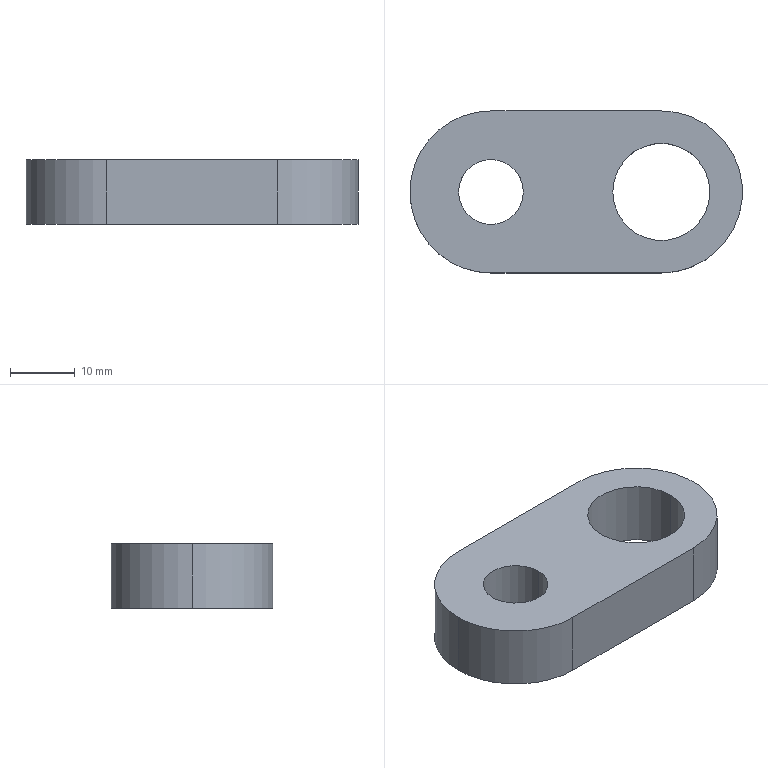Part | SolidWorks | features Extrusion 1 | 1 solid | 11 faces | box 51.31 x 25 x 10 mm | volume 8934 mm3 | cylinder 7 | plane 4 | commonest cylinder face diameters 25 x3 10 x2 15 x2
STEP:
#1=CARTESIAN_POINT('',(5.655,0.,10.));
#2=VERTEX_POINT('',#1);
#3=CARTESIAN_POINT('',(20.655,0.,10.));
#4=VERTEX_POINT('',#3);
#5=CARTESIAN_POINT('',(13.155,0.,10.));
#6=DIRECTION('',(0.,0.,1.));
#7=DIRECTION('',(1.,0.,0.));
#8=AXIS2_PLACEMENT_3D('',#5,#6,#7);
#9=CIRCLE('',#8,7.5);
#10=EDGE_CURVE('',#2,#4,#9,.T.);
#11=ORIENTED_EDGE('',*,*,#10,.T.);
#12=CARTESIAN_POINT('',(20.655,0.,0.));
#13=VERTEX_POINT('',#12);
#14=CARTESIAN_POINT('',(20.655,0.,10.));
#15=DIRECTION('',(0.,0.,-1.));
#16=VECTOR('',#15,1000.);
#17=LINE('',#14,#16);
#18=EDGE_CURVE('',#4,#13,#17,.T.);
#19=ORIENTED_EDGE('',*,*,#18,.T.);
#20=CARTESIAN_POINT('',(5.655,0.,0.));
#21=VERTEX_POINT('',#20);
#22=CARTESIAN_POINT('',(13.155,0.,0.));
#23=DIRECTION('',(0.,0.,1.));
#24=DIRECTION('',(1.,0.,0.));
#25=AXIS2_PLACEMENT_3D('',#22,#23,#24);
#26=CIRCLE('',#25,7.5);
#27=EDGE_CURVE('',#21,#13,#26,.T.);
#28=ORIENTED_EDGE('',*,*,#27,.F.);
#29=CARTESIAN_POINT('',(5.655,0.,10.));
#30=DIRECTION('',(0.,0.,-1.));
#31=VECTOR('',#30,1000.);
#32=LINE('',#29,#31);
#33=EDGE_CURVE('',#2,#21,#32,.T.);
#34=ORIENTED_EDGE('',*,*,#33,.F.);
#35=EDGE_LOOP('',(#11,#19,#28,#34));
#36=FACE_OUTER_BOUND('',#35,.T.);
#37=CARTESIAN_POINT('',(13.155,0.,10.));
#38=DIRECTION('',(0.,0.,-1.));
#39=DIRECTION('',(-1.,0.,0.));
#40=AXIS2_PLACEMENT_3D('',#37,#38,#39);
#41=CYLINDRICAL_SURFACE('',#40,7.5);
#42=ADVANCED_FACE('',(#36),#41,.F.);
#43=CARTESIAN_POINT('',(-18.155,0.,10.));
#44=VERTEX_POINT('',#43);
#45=CARTESIAN_POINT('',(-8.155,0.,10.));
#46=VERTEX_POINT('',#45);
#47=CARTESIAN_POINT('',(-13.155,0.,10.));
#48=DIRECTION('',(0.,0.,1.));
#49=DIRECTION('',(1.,0.,0.));
#50=AXIS2_PLACEMENT_3D('',#47,#48,#49);
#51=CIRCLE('',#50,5.);
#52=EDGE_CURVE('',#44,#46,#51,.T.);
#53=ORIENTED_EDGE('',*,*,#52,.T.);
#54=CARTESIAN_POINT('',(-8.155,0.,0.));
#55=VERTEX_POINT('',#54);
#56=CARTESIAN_POINT('',(-8.155,0.,10.));
#57=DIRECTION('',(0.,0.,-1.));
#58=VECTOR('',#57,1000.);
#59=LINE('',#56,#58);
#60=EDGE_CURVE('',#46,#55,#59,.T.);
#61=ORIENTED_EDGE('',*,*,#60,.T.);
#62=CARTESIAN_POINT('',(-18.155,0.,0.));
#63=VERTEX_POINT('',#62);
#64=CARTESIAN_POINT('',(-13.155,0.,0.));
#65=DIRECTION('',(0.,0.,1.));
#66=DIRECTION('',(1.,0.,0.));
#67=AXIS2_PLACEMENT_3D('',#64,#65,#66);
#68=CIRCLE('',#67,5.);
#69=EDGE_CURVE('',#63,#55,#68,.T.);
#70=ORIENTED_EDGE('',*,*,#69,.F.);
#71=CARTESIAN_POINT('',(-18.155,0.,10.));
#72=DIRECTION('',(0.,0.,-1.));
#73=VECTOR('',#72,1000.);
#74=LINE('',#71,#73);
#75=EDGE_CURVE('',#44,#63,#74,.T.);
#76=ORIENTED_EDGE('',*,*,#75,.F.);
#77=EDGE_LOOP('',(#53,#61,#70,#76));
#78=FACE_OUTER_BOUND('',#77,.T.);
#79=CARTESIAN_POINT('',(-13.155,0.,10.));
#80=DIRECTION('',(0.,0.,-1.));
#81=DIRECTION('',(-1.,0.,0.));
#82=AXIS2_PLACEMENT_3D('',#79,#80,#81);
#83=CYLINDRICAL_SURFACE('',#82,5.);
#84=ADVANCED_FACE('',(#78),#83,.F.);
#85=CARTESIAN_POINT('',(-25.655,0.,10.));
#86=VERTEX_POINT('',#85);
#87=CARTESIAN_POINT('',(-13.155,-12.5,10.));
#88=VERTEX_POINT('',#87);
#89=CARTESIAN_POINT('',(-13.155,0.,10.));
#90=DIRECTION('',(0.,0.,1.));
#91=DIRECTION('',(1.,0.,0.));
#92=AXIS2_PLACEMENT_3D('',#89,#90,#91);
#93=CIRCLE('',#92,12.5);
#94=EDGE_CURVE('',#86,#88,#93,.T.);
#95=ORIENTED_EDGE('',*,*,#94,.F.);
#96=CARTESIAN_POINT('',(-25.655,0.,0.));
#97=VERTEX_POINT('',#96);
#98=CARTESIAN_POINT('',(-25.655,0.,10.));
#99=DIRECTION('',(0.,0.,-1.));
#100=VECTOR('',#99,1000.);
#101=LINE('',#98,#100);
#102=EDGE_CURVE('',#86,#97,#101,.T.);
#103=ORIENTED_EDGE('',*,*,#102,.T.);
#104=CARTESIAN_POINT('',(-13.155,-12.5,0.));
#105=VERTEX_POINT('',#104);
#106=CARTESIAN_POINT('',(-13.155,0.,0.));
#107=DIRECTION('',(0.,0.,1.));
#108=DIRECTION('',(1.,0.,0.));
#109=AXIS2_PLACEMENT_3D('',#106,#107,#108);
#110=CIRCLE('',#109,12.5);
#111=EDGE_CURVE('',#97,#105,#110,.T.);
#112=ORIENTED_EDGE('',*,*,#111,.T.);
#113=CARTESIAN_POINT('',(-13.155,-12.5,10.));
#114=DIRECTION('',(0.,0.,-1.));
#115=VECTOR('',#114,1000.);
#116=LINE('',#113,#115);
#117=EDGE_CURVE('',#88,#105,#116,.T.);
#118=ORIENTED_EDGE('',*,*,#117,.F.);
#119=EDGE_LOOP('',(#95,#103,#112,#118));
#120=FACE_OUTER_BOUND('',#119,.T.);
#121=CARTESIAN_POINT('',(-13.155,0.,10.));
#122=DIRECTION('',(0.,0.,-1.));
#123=DIRECTION('',(-1.,0.,0.));
#124=AXIS2_PLACEMENT_3D('',#121,#122,#123);
#125=CYLINDRICAL_SURFACE('',#124,12.5);
#126=ADVANCED_FACE('',(#120),#125,.T.);
#127=ORIENTED_EDGE('',*,*,#52,.F.);
#128=CARTESIAN_POINT('',(-13.155,0.,10.));
#129=DIRECTION('',(0.,0.,1.));
#130=DIRECTION('',(1.,0.,0.));
#131=AXIS2_PLACEMENT_3D('',#128,#129,#130);
#132=CIRCLE('',#131,5.);
#133=EDGE_CURVE('',#46,#44,#132,.T.);
#134=ORIENTED_EDGE('',*,*,#133,.F.);
#135=EDGE_LOOP('',(#127,#134));
#136=FACE_BOUND('',#135,.T.);
#137=CARTESIAN_POINT('',(-13.155,12.5,10.));
#138=VERTEX_POINT('',#137);
#139=CARTESIAN_POINT('',(-13.155,0.,10.));
#140=DIRECTION('',(0.,0.,1.));
#141=DIRECTION('',(1.,0.,0.));
#142=AXIS2_PLACEMENT_3D('',#139,#140,#141);
#143=CIRCLE('',#142,12.5);
#144=EDGE_CURVE('',#138,#86,#143,.T.);
#145=ORIENTED_EDGE('',*,*,#144,.T.);
#146=ORIENTED_EDGE('',*,*,#94,.T.);
#147=CARTESIAN_POINT('',(13.155,-12.5,10.));
#148=VERTEX_POINT('',#147);
#149=CARTESIAN_POINT('',(-13.155,-12.5,10.));
#150=DIRECTION('',(1.,0.,0.));
#151=VECTOR('',#150,1000.);
#152=LINE('',#149,#151);
#153=EDGE_CURVE('',#88,#148,#152,.T.);
#154=ORIENTED_EDGE('',*,*,#153,.T.);
#155=CARTESIAN_POINT('',(13.155,12.5,10.));
#156=VERTEX_POINT('',#155);
#157=CARTESIAN_POINT('',(13.155,0.,10.));
#158=DIRECTION('',(0.,0.,1.));
#159=DIRECTION('',(1.,0.,0.));
#160=AXIS2_PLACEMENT_3D('',#157,#158,#159);
#161=CIRCLE('',#160,12.5);
#162=EDGE_CURVE('',#148,#156,#161,.T.);
#163=ORIENTED_EDGE('',*,*,#162,.T.);
#164=CARTESIAN_POINT('',(-13.155,12.5,10.));
#165=DIRECTION('',(-1.,0.,0.));
#166=VECTOR('',#165,1000.);
#167=LINE('',#164,#166);
#168=EDGE_CURVE('',#156,#138,#167,.T.);
#169=ORIENTED_EDGE('',*,*,#168,.T.);
#170=EDGE_LOOP('',(#145,#146,#154,#163,#169));
#171=FACE_OUTER_BOUND('',#170,.T.);
#172=ORIENTED_EDGE('',*,*,#10,.F.);
#173=CARTESIAN_POINT('',(13.155,0.,10.));
#174=DIRECTION('',(0.,0.,1.));
#175=DIRECTION('',(1.,0.,0.));
#176=AXIS2_PLACEMENT_3D('',#173,#174,#175);
#177=CIRCLE('',#176,7.5);
#178=EDGE_CURVE('',#4,#2,#177,.T.);
#179=ORIENTED_EDGE('',*,*,#178,.F.);
#180=EDGE_LOOP('',(#172,#179));
#181=FACE_BOUND('',#180,.T.);
#182=CARTESIAN_POINT('',(-13.155,0.,10.));
#183=DIRECTION('',(0.,0.,1.));
#184=DIRECTION('',(1.,0.,0.));
#185=AXIS2_PLACEMENT_3D('',#182,#183,#184);
#186=PLANE('',#185);
#187=ADVANCED_FACE('',(#136,#171,#181),#186,.T.);
#188=CARTESIAN_POINT('',(-13.155,12.5,0.));
#189=VERTEX_POINT('',#188);
#190=CARTESIAN_POINT('',(-13.155,0.,0.));
#191=DIRECTION('',(0.,0.,1.));
#192=DIRECTION('',(1.,0.,0.));
#193=AXIS2_PLACEMENT_3D('',#190,#191,#192);
#194=CIRCLE('',#193,12.5);
#195=EDGE_CURVE('',#189,#97,#194,.T.);
#196=ORIENTED_EDGE('',*,*,#195,.F.);
#197=CARTESIAN_POINT('',(13.155,12.5,0.));
#198=VERTEX_POINT('',#197);
#199=CARTESIAN_POINT('',(-13.155,12.5,0.));
#200=DIRECTION('',(-1.,0.,0.));
#201=VECTOR('',#200,1000.);
#202=LINE('',#199,#201);
#203=EDGE_CURVE('',#198,#189,#202,.T.);
#204=ORIENTED_EDGE('',*,*,#203,.F.);
#205=CARTESIAN_POINT('',(13.155,-12.5,0.));
#206=VERTEX_POINT('',#205);
#207=CARTESIAN_POINT('',(13.155,0.,0.));
#208=DIRECTION('',(0.,0.,1.));
#209=DIRECTION('',(1.,0.,0.));
#210=AXIS2_PLACEMENT_3D('',#207,#208,#209);
#211=CIRCLE('',#210,12.5);
#212=EDGE_CURVE('',#206,#198,#211,.T.);
#213=ORIENTED_EDGE('',*,*,#212,.F.);
#214=CARTESIAN_POINT('',(-13.155,-12.5,0.));
#215=DIRECTION('',(1.,0.,0.));
#216=VECTOR('',#215,1000.);
#217=LINE('',#214,#216);
#218=EDGE_CURVE('',#105,#206,#217,.T.);
#219=ORIENTED_EDGE('',*,*,#218,.F.);
#220=ORIENTED_EDGE('',*,*,#111,.F.);
#221=EDGE_LOOP('',(#196,#204,#213,#219,#220));
#222=FACE_OUTER_BOUND('',#221,.T.);
#223=ORIENTED_EDGE('',*,*,#69,.T.);
#224=CARTESIAN_POINT('',(-13.155,0.,0.));
#225=DIRECTION('',(0.,0.,1.));
#226=DIRECTION('',(1.,0.,0.));
#227=AXIS2_PLACEMENT_3D('',#224,#225,#226);
#228=CIRCLE('',#227,5.);
#229=EDGE_CURVE('',#55,#63,#228,.T.);
#230=ORIENTED_EDGE('',*,*,#229,.T.);
#231=EDGE_LOOP('',(#223,#230));
#232=FACE_BOUND('',#231,.T.);
#233=ORIENTED_EDGE('',*,*,#27,.T.);
#234=CARTESIAN_POINT('',(13.155,0.,0.));
#235=DIRECTION('',(0.,0.,1.));
#236=DIRECTION('',(1.,0.,0.));
#237=AXIS2_PLACEMENT_3D('',#234,#235,#236);
#238=CIRCLE('',#237,7.5);
#239=EDGE_CURVE('',#13,#21,#238,.T.);
#240=ORIENTED_EDGE('',*,*,#239,.T.);
#241=EDGE_LOOP('',(#233,#240));
#242=FACE_BOUND('',#241,.T.);
#243=CARTESIAN_POINT('',(-13.155,0.,0.));
#244=DIRECTION('',(0.,0.,1.));
#245=DIRECTION('',(1.,0.,0.));
#246=AXIS2_PLACEMENT_3D('',#243,#244,#245);
#247=PLANE('',#246);
#248=ADVANCED_FACE('',(#222,#232,#242),#247,.F.);
#249=ORIENTED_EDGE('',*,*,#102,.F.);
#250=ORIENTED_EDGE('',*,*,#144,.F.);
#251=CARTESIAN_POINT('',(-13.155,12.5,10.));
#252=DIRECTION('',(0.,0.,-1.));
#253=VECTOR('',#252,1000.);
#254=LINE('',#251,#253);
#255=EDGE_CURVE('',#138,#189,#254,.T.);
#256=ORIENTED_EDGE('',*,*,#255,.T.);
#257=ORIENTED_EDGE('',*,*,#195,.T.);
#258=EDGE_LOOP('',(#249,#250,#256,#257));
#259=FACE_OUTER_BOUND('',#258,.T.);
#260=CARTESIAN_POINT('',(-13.155,0.,10.));
#261=DIRECTION('',(0.,0.,-1.));
#262=DIRECTION('',(-1.,0.,0.));
#263=AXIS2_PLACEMENT_3D('',#260,#261,#262);
#264=CYLINDRICAL_SURFACE('',#263,12.5);
#265=ADVANCED_FACE('',(#259),#264,.T.);
#266=ORIENTED_EDGE('',*,*,#218,.T.);
#267=CARTESIAN_POINT('',(13.155,-12.5,10.));
#268=DIRECTION('',(0.,0.,-1.));
#269=VECTOR('',#268,1000.);
#270=LINE('',#267,#269);
#271=EDGE_CURVE('',#148,#206,#270,.T.);
#272=ORIENTED_EDGE('',*,*,#271,.F.);
#273=ORIENTED_EDGE('',*,*,#153,.F.);
#274=ORIENTED_EDGE('',*,*,#117,.T.);
#275=EDGE_LOOP('',(#266,#272,#273,#274));
#276=FACE_OUTER_BOUND('',#275,.T.);
#277=CARTESIAN_POINT('',(-13.155,-12.5,10.));
#278=DIRECTION('',(0.,1.,0.));
#279=DIRECTION('',(0.,0.,1.));
#280=AXIS2_PLACEMENT_3D('',#277,#278,#279);
#281=PLANE('',#280);
#282=ADVANCED_FACE('',(#276),#281,.F.);
#283=ORIENTED_EDGE('',*,*,#212,.T.);
#284=CARTESIAN_POINT('',(13.155,12.5,10.));
#285=DIRECTION('',(0.,0.,-1.));
#286=VECTOR('',#285,1000.);
#287=LINE('',#284,#286);
#288=EDGE_CURVE('',#156,#198,#287,.T.);
#289=ORIENTED_EDGE('',*,*,#288,.F.);
#290=ORIENTED_EDGE('',*,*,#162,.F.);
#291=ORIENTED_EDGE('',*,*,#271,.T.);
#292=EDGE_LOOP('',(#283,#289,#290,#291));
#293=FACE_OUTER_BOUND('',#292,.T.);
#294=CARTESIAN_POINT('',(13.155,0.,10.));
#295=DIRECTION('',(0.,0.,-1.));
#296=DIRECTION('',(-1.,0.,0.));
#297=AXIS2_PLACEMENT_3D('',#294,#295,#296);
#298=CYLINDRICAL_SURFACE('',#297,12.5);
#299=ADVANCED_FACE('',(#293),#298,.T.);
#300=ORIENTED_EDGE('',*,*,#203,.T.);
#301=ORIENTED_EDGE('',*,*,#255,.F.);
#302=ORIENTED_EDGE('',*,*,#168,.F.);
#303=ORIENTED_EDGE('',*,*,#288,.T.);
#304=EDGE_LOOP('',(#300,#301,#302,#303));
#305=FACE_OUTER_BOUND('',#304,.T.);
#306=CARTESIAN_POINT('',(-13.155,12.5,10.));
#307=DIRECTION('',(0.,-1.,0.));
#308=DIRECTION('',(0.,0.,-1.));
#309=AXIS2_PLACEMENT_3D('',#306,#307,#308);
#310=PLANE('',#309);
#311=ADVANCED_FACE('',(#305),#310,.F.);
#312=ORIENTED_EDGE('',*,*,#60,.F.);
#313=ORIENTED_EDGE('',*,*,#133,.T.);
#314=ORIENTED_EDGE('',*,*,#75,.T.);
#315=ORIENTED_EDGE('',*,*,#229,.F.);
#316=EDGE_LOOP('',(#312,#313,#314,#315));
#317=FACE_OUTER_BOUND('',#316,.T.);
#318=CARTESIAN_POINT('',(-13.155,0.,10.));
#319=DIRECTION('',(0.,0.,-1.));
#320=DIRECTION('',(-1.,0.,0.));
#321=AXIS2_PLACEMENT_3D('',#318,#319,#320);
#322=CYLINDRICAL_SURFACE('',#321,5.);
#323=ADVANCED_FACE('',(#317),#322,.F.);
#324=ORIENTED_EDGE('',*,*,#18,.F.);
#325=ORIENTED_EDGE('',*,*,#178,.T.);
#326=ORIENTED_EDGE('',*,*,#33,.T.);
#327=ORIENTED_EDGE('',*,*,#239,.F.);
#328=EDGE_LOOP('',(#324,#325,#326,#327));
#329=FACE_OUTER_BOUND('',#328,.T.);
#330=CARTESIAN_POINT('',(13.155,0.,10.));
#331=DIRECTION('',(0.,0.,-1.));
#332=DIRECTION('',(-1.,0.,0.));
#333=AXIS2_PLACEMENT_3D('',#330,#331,#332);
#334=CYLINDRICAL_SURFACE('',#333,7.5);
#335=ADVANCED_FACE('',(#329),#334,.F.);
#336=CLOSED_SHELL('',(#42,#84,#126,#187,#248,#265,#282,#299,#311,#323,#335));
#337=MANIFOLD_SOLID_BREP('',#336);
#338=CARTESIAN_POINT('',(0.,0.,0.));
#339=DIRECTION('',(0.,0.,1.));
#340=DIRECTION('',(1.,0.,0.));
#341=AXIS2_PLACEMENT_3D('',#338,#339,#340);
#342=(LENGTH_UNIT()NAMED_UNIT(*)SI_UNIT(.MILLI.,.METRE.));
#343=UNCERTAINTY_MEASURE_WITH_UNIT(LENGTH_MEASURE(0.00001),#342,'','');
#344=(NAMED_UNIT(*)PLANE_ANGLE_UNIT()SI_UNIT($,.RADIAN.));
#345=(NAMED_UNIT(*)SI_UNIT($,.STERADIAN.)SOLID_ANGLE_UNIT());
#346=(GEOMETRIC_REPRESENTATION_CONTEXT(3)GLOBAL_UNCERTAINTY_ASSIGNED_CONTEXT((#343))GLOBAL_UNIT_ASSIGNED_CONTEXT((#342,#344,#345))REPRESENTATION_CONTEXT('',''));
#347=ADVANCED_BREP_SHAPE_REPRESENTATION('',(#337,#341),#346);